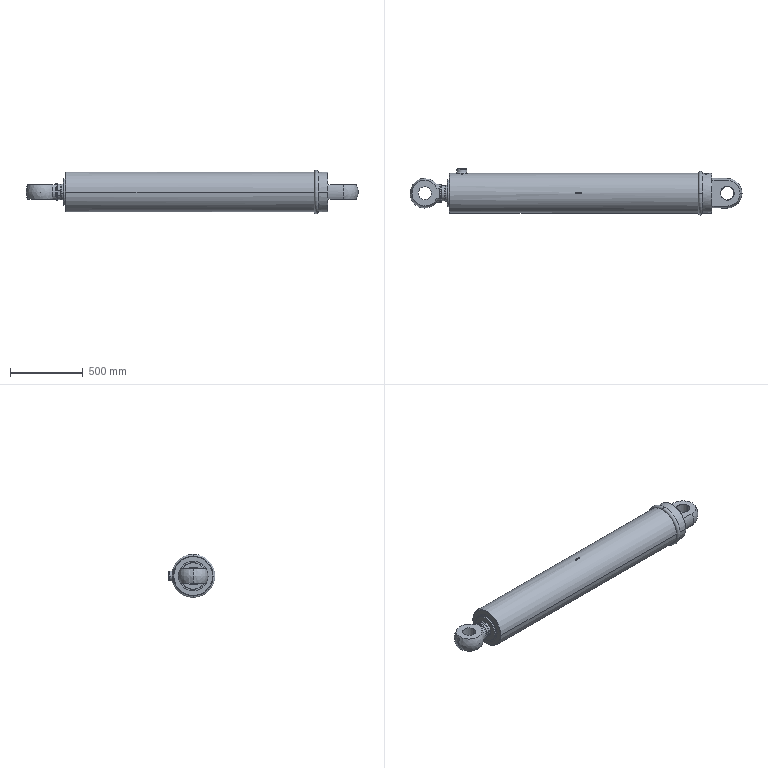Part | SolidWorks | 4 solids | 704 faces | box 2283 x 316.65 x 300.3 mm | volume 112052939 mm3 | plane 471 | cylinder 94 | spline 87 | cone 46 | sphere 4 | torus 2 | commonest cylinder face diameters 273.2 x48 273 x11 39.835 x4 81.753 x4 110 x4 90 x3